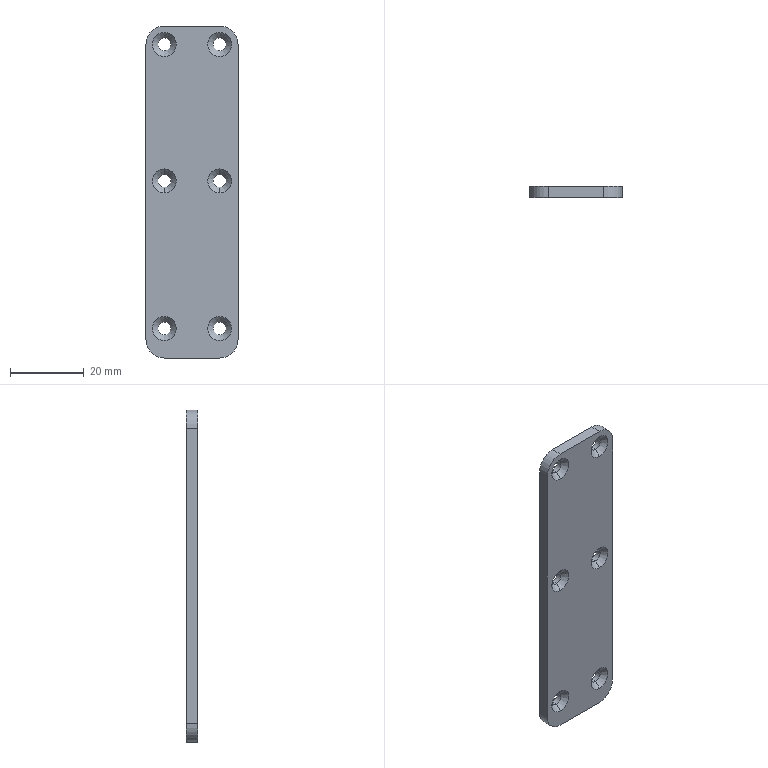Part | STEP file | 0246_210_Plate | 1 solid | 34 faces | box 25 x 3 x 90 mm | volume 6417 mm3 | cylinder 16 | cone 12 | plane 6 | commonest cylinder face diameters 3.5 x12 10 x4